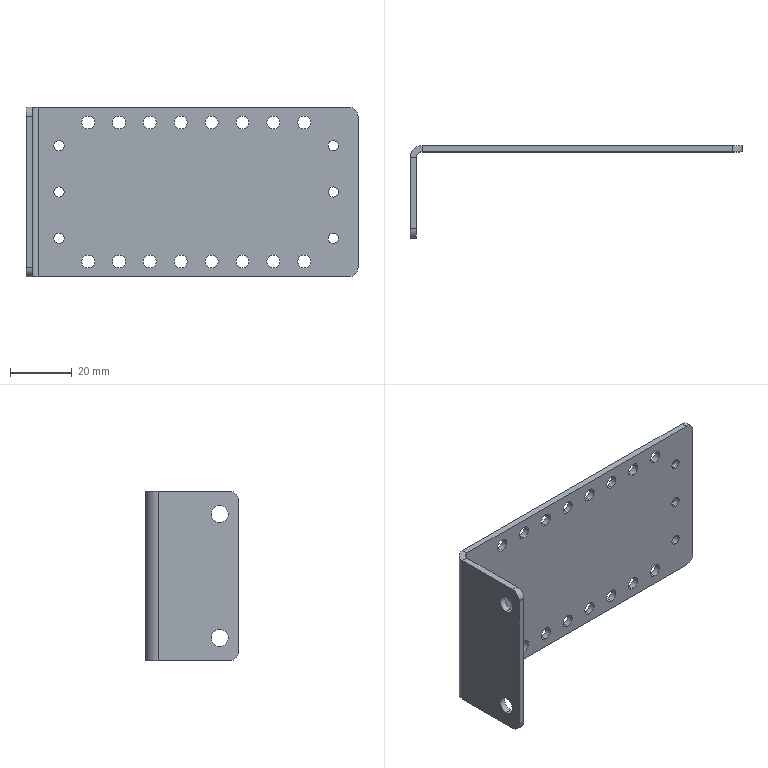Part | SolidWorks | features HoleWzd 3, Fillet 1, FlatPattern 1, SMBaseFlange 1, SheetMetal 1 | 1 solid | 66 faces | box 107.5 x 30 x 55 mm | volume 14107 mm3 | cylinder 54 | plane 12 | commonest cylinder face diameters 4.2 x32 3.3 x12 5.5 x4 6 x4 4 x1 8 x1